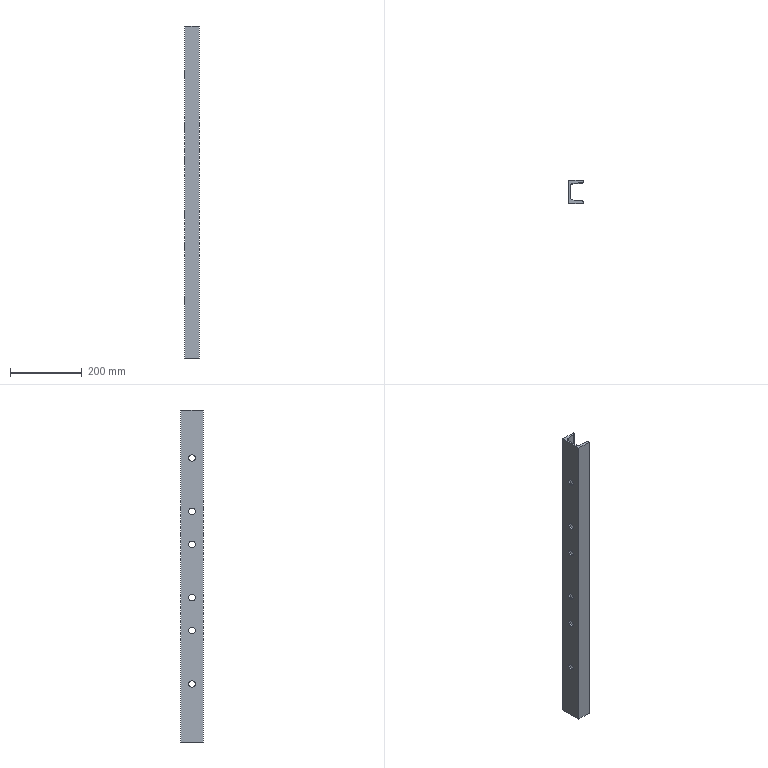Part | STEP file | 750038456 | 1 solid | 26 faces | box 40 x 63 x 924 mm | volume 773051 mm3 | cylinder 16 | plane 10 | commonest cylinder face diameters 18 x12 7.6 x2 15 x2
STEP:
#1=CARTESIAN_POINT('',(4.8,31.5,170.754));
#2=VERTEX_POINT('',#1);
#3=CARTESIAN_POINT('',(4.8,31.5,188.754));
#4=VERTEX_POINT('',#3);
#5=CARTESIAN_POINT('',(4.8,31.5,179.754));
#6=DIRECTION('',(-1.,0.,0.));
#7=DIRECTION('',(0.,0.,1.));
#8=AXIS2_PLACEMENT_3D('',#5,#6,#7);
#9=CIRCLE('',#8,9.);
#10=EDGE_CURVE('',#2,#4,#9,.T.);
#11=ORIENTED_EDGE('',*,*,#10,.F.);
#12=CARTESIAN_POINT('',(0.,31.5,170.754));
#13=VERTEX_POINT('',#12);
#14=CARTESIAN_POINT('',(44.,31.5,170.754));
#15=DIRECTION('',(-1.,0.,0.));
#16=VECTOR('',#15,1000.);
#17=LINE('',#14,#16);
#18=EDGE_CURVE('',#2,#13,#17,.T.);
#19=ORIENTED_EDGE('',*,*,#18,.T.);
#20=CARTESIAN_POINT('',(0.,31.5,188.754));
#21=VERTEX_POINT('',#20);
#22=CARTESIAN_POINT('',(0.,31.5,179.754));
#23=DIRECTION('',(-1.,0.,0.));
#24=DIRECTION('',(0.,0.,1.));
#25=AXIS2_PLACEMENT_3D('',#22,#23,#24);
#26=CIRCLE('',#25,9.);
#27=EDGE_CURVE('',#13,#21,#26,.T.);
#28=ORIENTED_EDGE('',*,*,#27,.T.);
#29=CARTESIAN_POINT('',(44.,31.5,188.754));
#30=DIRECTION('',(-1.,0.,0.));
#31=VECTOR('',#30,1000.);
#32=LINE('',#29,#31);
#33=EDGE_CURVE('',#4,#21,#32,.T.);
#34=ORIENTED_EDGE('',*,*,#33,.F.);
#35=EDGE_LOOP('',(#11,#19,#28,#34));
#36=FACE_OUTER_BOUND('',#35,.T.);
#37=CARTESIAN_POINT('',(44.,31.5,179.754));
#38=DIRECTION('',(-1.,0.,0.));
#39=DIRECTION('',(0.,0.,1.));
#40=AXIS2_PLACEMENT_3D('',#37,#38,#39);
#41=CYLINDRICAL_SURFACE('',#40,9.);
#42=ADVANCED_FACE('',(#36),#41,.F.);
#43=CARTESIAN_POINT('',(4.8,31.5,79.246));
#44=VERTEX_POINT('',#43);
#45=CARTESIAN_POINT('',(4.8,31.5,97.246));
#46=VERTEX_POINT('',#45);
#47=CARTESIAN_POINT('',(4.8,31.5,88.246));
#48=DIRECTION('',(-1.,0.,0.));
#49=DIRECTION('',(0.,0.,1.));
#50=AXIS2_PLACEMENT_3D('',#47,#48,#49);
#51=CIRCLE('',#50,9.);
#52=EDGE_CURVE('',#44,#46,#51,.T.);
#53=ORIENTED_EDGE('',*,*,#52,.F.);
#54=CARTESIAN_POINT('',(0.,31.5,79.246));
#55=VERTEX_POINT('',#54);
#56=CARTESIAN_POINT('',(44.,31.5,79.246));
#57=DIRECTION('',(-1.,0.,0.));
#58=VECTOR('',#57,1000.);
#59=LINE('',#56,#58);
#60=EDGE_CURVE('',#44,#55,#59,.T.);
#61=ORIENTED_EDGE('',*,*,#60,.T.);
#62=CARTESIAN_POINT('',(0.,31.5,97.246));
#63=VERTEX_POINT('',#62);
#64=CARTESIAN_POINT('',(0.,31.5,88.246));
#65=DIRECTION('',(-1.,0.,0.));
#66=DIRECTION('',(0.,0.,1.));
#67=AXIS2_PLACEMENT_3D('',#64,#65,#66);
#68=CIRCLE('',#67,9.);
#69=EDGE_CURVE('',#55,#63,#68,.T.);
#70=ORIENTED_EDGE('',*,*,#69,.T.);
#71=CARTESIAN_POINT('',(44.,31.5,97.246));
#72=DIRECTION('',(-1.,0.,0.));
#73=VECTOR('',#72,1000.);
#74=LINE('',#71,#73);
#75=EDGE_CURVE('',#46,#63,#74,.T.);
#76=ORIENTED_EDGE('',*,*,#75,.F.);
#77=EDGE_LOOP('',(#53,#61,#70,#76));
#78=FACE_OUTER_BOUND('',#77,.T.);
#79=CARTESIAN_POINT('',(44.,31.5,88.246));
#80=DIRECTION('',(-1.,0.,0.));
#81=DIRECTION('',(0.,0.,1.));
#82=AXIS2_PLACEMENT_3D('',#79,#80,#81);
#83=CYLINDRICAL_SURFACE('',#82,9.);
#84=ADVANCED_FACE('',(#78),#83,.F.);
#85=CARTESIAN_POINT('',(4.8,31.5,-160.754));
#86=VERTEX_POINT('',#85);
#87=CARTESIAN_POINT('',(4.8,31.5,-142.754));
#88=VERTEX_POINT('',#87);
#89=CARTESIAN_POINT('',(4.8,31.5,-151.754));
#90=DIRECTION('',(-1.,0.,0.));
#91=DIRECTION('',(0.,0.,1.));
#92=AXIS2_PLACEMENT_3D('',#89,#90,#91);
#93=CIRCLE('',#92,9.);
#94=EDGE_CURVE('',#86,#88,#93,.T.);
#95=ORIENTED_EDGE('',*,*,#94,.F.);
#96=CARTESIAN_POINT('',(0.,31.5,-160.754));
#97=VERTEX_POINT('',#96);
#98=CARTESIAN_POINT('',(44.,31.5,-160.754));
#99=DIRECTION('',(-1.,0.,0.));
#100=VECTOR('',#99,1000.);
#101=LINE('',#98,#100);
#102=EDGE_CURVE('',#86,#97,#101,.T.);
#103=ORIENTED_EDGE('',*,*,#102,.T.);
#104=CARTESIAN_POINT('',(0.,31.5,-142.754));
#105=VERTEX_POINT('',#104);
#106=CARTESIAN_POINT('',(0.,31.5,-151.754));
#107=DIRECTION('',(-1.,0.,0.));
#108=DIRECTION('',(0.,0.,1.));
#109=AXIS2_PLACEMENT_3D('',#106,#107,#108);
#110=CIRCLE('',#109,9.);
#111=EDGE_CURVE('',#97,#105,#110,.T.);
#112=ORIENTED_EDGE('',*,*,#111,.T.);
#113=CARTESIAN_POINT('',(44.,31.5,-142.754));
#114=DIRECTION('',(-1.,0.,0.));
#115=VECTOR('',#114,1000.);
#116=LINE('',#113,#115);
#117=EDGE_CURVE('',#88,#105,#116,.T.);
#118=ORIENTED_EDGE('',*,*,#117,.F.);
#119=EDGE_LOOP('',(#95,#103,#112,#118));
#120=FACE_OUTER_BOUND('',#119,.T.);
#121=CARTESIAN_POINT('',(44.,31.5,-151.754));
#122=DIRECTION('',(-1.,0.,0.));
#123=DIRECTION('',(0.,0.,1.));
#124=AXIS2_PLACEMENT_3D('',#121,#122,#123);
#125=CYLINDRICAL_SURFACE('',#124,9.);
#126=ADVANCED_FACE('',(#120),#125,.F.);
#127=CARTESIAN_POINT('',(4.8,31.5,-309.246));
#128=VERTEX_POINT('',#127);
#129=CARTESIAN_POINT('',(4.8,31.5,-291.246));
#130=VERTEX_POINT('',#129);
#131=CARTESIAN_POINT('',(4.8,31.5,-300.246));
#132=DIRECTION('',(-1.,0.,0.));
#133=DIRECTION('',(0.,0.,1.));
#134=AXIS2_PLACEMENT_3D('',#131,#132,#133);
#135=CIRCLE('',#134,9.);
#136=EDGE_CURVE('',#128,#130,#135,.T.);
#137=ORIENTED_EDGE('',*,*,#136,.F.);
#138=CARTESIAN_POINT('',(0.,31.5,-309.246));
#139=VERTEX_POINT('',#138);
#140=CARTESIAN_POINT('',(44.,31.5,-309.246));
#141=DIRECTION('',(-1.,0.,0.));
#142=VECTOR('',#141,1000.);
#143=LINE('',#140,#142);
#144=EDGE_CURVE('',#128,#139,#143,.T.);
#145=ORIENTED_EDGE('',*,*,#144,.T.);
#146=CARTESIAN_POINT('',(0.,31.5,-291.246));
#147=VERTEX_POINT('',#146);
#148=CARTESIAN_POINT('',(0.,31.5,-300.246));
#149=DIRECTION('',(-1.,0.,0.));
#150=DIRECTION('',(0.,0.,1.));
#151=AXIS2_PLACEMENT_3D('',#148,#149,#150);
#152=CIRCLE('',#151,9.);
#153=EDGE_CURVE('',#139,#147,#152,.T.);
#154=ORIENTED_EDGE('',*,*,#153,.T.);
#155=CARTESIAN_POINT('',(44.,31.5,-291.246));
#156=DIRECTION('',(-1.,0.,0.));
#157=VECTOR('',#156,1000.);
#158=LINE('',#155,#157);
#159=EDGE_CURVE('',#130,#147,#158,.T.);
#160=ORIENTED_EDGE('',*,*,#159,.F.);
#161=EDGE_LOOP('',(#137,#145,#154,#160));
#162=FACE_OUTER_BOUND('',#161,.T.);
#163=CARTESIAN_POINT('',(44.,31.5,-300.246));
#164=DIRECTION('',(-1.,0.,0.));
#165=DIRECTION('',(0.,0.,1.));
#166=AXIS2_PLACEMENT_3D('',#163,#164,#165);
#167=CYLINDRICAL_SURFACE('',#166,9.);
#168=ADVANCED_FACE('',(#162),#167,.F.);
#169=CARTESIAN_POINT('',(4.8,31.5,-69.246));
#170=VERTEX_POINT('',#169);
#171=CARTESIAN_POINT('',(4.8,31.5,-51.246));
#172=VERTEX_POINT('',#171);
#173=CARTESIAN_POINT('',(4.8,31.5,-60.246));
#174=DIRECTION('',(-1.,0.,0.));
#175=DIRECTION('',(0.,0.,1.));
#176=AXIS2_PLACEMENT_3D('',#173,#174,#175);
#177=CIRCLE('',#176,9.);
#178=EDGE_CURVE('',#170,#172,#177,.T.);
#179=ORIENTED_EDGE('',*,*,#178,.F.);
#180=CARTESIAN_POINT('',(0.,31.5,-69.246));
#181=VERTEX_POINT('',#180);
#182=CARTESIAN_POINT('',(44.,31.5,-69.246));
#183=DIRECTION('',(-1.,0.,0.));
#184=VECTOR('',#183,1000.);
#185=LINE('',#182,#184);
#186=EDGE_CURVE('',#170,#181,#185,.T.);
#187=ORIENTED_EDGE('',*,*,#186,.T.);
#188=CARTESIAN_POINT('',(0.,31.5,-51.246));
#189=VERTEX_POINT('',#188);
#190=CARTESIAN_POINT('',(0.,31.5,-60.246));
#191=DIRECTION('',(-1.,0.,0.));
#192=DIRECTION('',(0.,0.,1.));
#193=AXIS2_PLACEMENT_3D('',#190,#191,#192);
#194=CIRCLE('',#193,9.);
#195=EDGE_CURVE('',#181,#189,#194,.T.);
#196=ORIENTED_EDGE('',*,*,#195,.T.);
#197=CARTESIAN_POINT('',(44.,31.5,-51.246));
#198=DIRECTION('',(-1.,0.,0.));
#199=VECTOR('',#198,1000.);
#200=LINE('',#197,#199);
#201=EDGE_CURVE('',#172,#189,#200,.T.);
#202=ORIENTED_EDGE('',*,*,#201,.F.);
#203=EDGE_LOOP('',(#179,#187,#196,#202));
#204=FACE_OUTER_BOUND('',#203,.T.);
#205=CARTESIAN_POINT('',(44.,31.5,-60.246));
#206=DIRECTION('',(-1.,0.,0.));
#207=DIRECTION('',(0.,0.,1.));
#208=AXIS2_PLACEMENT_3D('',#205,#206,#207);
#209=CYLINDRICAL_SURFACE('',#208,9.);
#210=ADVANCED_FACE('',(#204),#209,.F.);
#211=CARTESIAN_POINT('',(4.8,31.5,319.246));
#212=VERTEX_POINT('',#211);
#213=CARTESIAN_POINT('',(4.8,31.5,337.246));
#214=VERTEX_POINT('',#213);
#215=CARTESIAN_POINT('',(4.8,31.5,328.246));
#216=DIRECTION('',(-1.,0.,0.));
#217=DIRECTION('',(0.,0.,1.));
#218=AXIS2_PLACEMENT_3D('',#215,#216,#217);
#219=CIRCLE('',#218,9.);
#220=EDGE_CURVE('',#212,#214,#219,.T.);
#221=ORIENTED_EDGE('',*,*,#220,.F.);
#222=CARTESIAN_POINT('',(0.,31.5,319.246));
#223=VERTEX_POINT('',#222);
#224=CARTESIAN_POINT('',(44.,31.5,319.246));
#225=DIRECTION('',(-1.,0.,0.));
#226=VECTOR('',#225,1000.);
#227=LINE('',#224,#226);
#228=EDGE_CURVE('',#212,#223,#227,.T.);
#229=ORIENTED_EDGE('',*,*,#228,.T.);
#230=CARTESIAN_POINT('',(0.,31.5,337.246));
#231=VERTEX_POINT('',#230);
#232=CARTESIAN_POINT('',(0.,31.5,328.246));
#233=DIRECTION('',(-1.,0.,0.));
#234=DIRECTION('',(0.,0.,1.));
#235=AXIS2_PLACEMENT_3D('',#232,#233,#234);
#236=CIRCLE('',#235,9.);
#237=EDGE_CURVE('',#223,#231,#236,.T.);
#238=ORIENTED_EDGE('',*,*,#237,.T.);
#239=CARTESIAN_POINT('',(44.,31.5,337.246));
#240=DIRECTION('',(-1.,0.,0.));
#241=VECTOR('',#240,1000.);
#242=LINE('',#239,#241);
#243=EDGE_CURVE('',#214,#231,#242,.T.);
#244=ORIENTED_EDGE('',*,*,#243,.F.);
#245=EDGE_LOOP('',(#221,#229,#238,#244));
#246=FACE_OUTER_BOUND('',#245,.T.);
#247=CARTESIAN_POINT('',(44.,31.5,328.246));
#248=DIRECTION('',(-1.,0.,0.));
#249=DIRECTION('',(0.,0.,1.));
#250=AXIS2_PLACEMENT_3D('',#247,#248,#249);
#251=CYLINDRICAL_SURFACE('',#250,9.);
#252=ADVANCED_FACE('',(#246),#251,.F.);
#253=CARTESIAN_POINT('',(0.,0.,462.));
#254=VERTEX_POINT('',#253);
#255=CARTESIAN_POINT('',(0.,0.,-462.));
#256=VERTEX_POINT('',#255);
#257=CARTESIAN_POINT('',(0.,0.,462.));
#258=DIRECTION('',(0.,0.,-1.));
#259=VECTOR('',#258,1000.);
#260=LINE('',#257,#259);
#261=EDGE_CURVE('',#254,#256,#260,.T.);
#262=ORIENTED_EDGE('',*,*,#261,.F.);
#263=CARTESIAN_POINT('',(0.,63.,462.));
#264=VERTEX_POINT('',#263);
#265=CARTESIAN_POINT('',(0.,63.,462.));
#266=DIRECTION('',(0.,-1.,0.));
#267=VECTOR('',#266,1000.);
#268=LINE('',#265,#267);
#269=EDGE_CURVE('',#264,#254,#268,.T.);
#270=ORIENTED_EDGE('',*,*,#269,.F.);
#271=CARTESIAN_POINT('',(0.,63.,-462.));
#272=VERTEX_POINT('',#271);
#273=CARTESIAN_POINT('',(0.,63.,462.));
#274=DIRECTION('',(0.,0.,1.));
#275=VECTOR('',#274,1000.);
#276=LINE('',#273,#275);
#277=EDGE_CURVE('',#272,#264,#276,.T.);
#278=ORIENTED_EDGE('',*,*,#277,.F.);
#279=CARTESIAN_POINT('',(0.,63.,-462.));
#280=DIRECTION('',(0.,1.,0.));
#281=VECTOR('',#280,1000.);
#282=LINE('',#279,#281);
#283=EDGE_CURVE('',#256,#272,#282,.T.);
#284=ORIENTED_EDGE('',*,*,#283,.F.);
#285=EDGE_LOOP('',(#262,#270,#278,#284));
#286=FACE_OUTER_BOUND('',#285,.T.);
#287=CARTESIAN_POINT('',(0.,31.5,179.754));
#288=DIRECTION('',(-1.,0.,0.));
#289=DIRECTION('',(0.,0.,1.));
#290=AXIS2_PLACEMENT_3D('',#287,#288,#289);
#291=CIRCLE('',#290,9.);
#292=EDGE_CURVE('',#21,#13,#291,.T.);
#293=ORIENTED_EDGE('',*,*,#292,.F.);
#294=ORIENTED_EDGE('',*,*,#27,.F.);
#295=EDGE_LOOP('',(#293,#294));
#296=FACE_BOUND('',#295,.T.);
#297=CARTESIAN_POINT('',(0.,31.5,88.246));
#298=DIRECTION('',(-1.,0.,0.));
#299=DIRECTION('',(0.,0.,1.));
#300=AXIS2_PLACEMENT_3D('',#297,#298,#299);
#301=CIRCLE('',#300,9.);
#302=EDGE_CURVE('',#63,#55,#301,.T.);
#303=ORIENTED_EDGE('',*,*,#302,.F.);
#304=ORIENTED_EDGE('',*,*,#69,.F.);
#305=EDGE_LOOP('',(#303,#304));
#306=FACE_BOUND('',#305,.T.);
#307=CARTESIAN_POINT('',(0.,31.5,-151.754));
#308=DIRECTION('',(-1.,0.,0.));
#309=DIRECTION('',(0.,0.,1.));
#310=AXIS2_PLACEMENT_3D('',#307,#308,#309);
#311=CIRCLE('',#310,9.);
#312=EDGE_CURVE('',#105,#97,#311,.T.);
#313=ORIENTED_EDGE('',*,*,#312,.F.);
#314=ORIENTED_EDGE('',*,*,#111,.F.);
#315=EDGE_LOOP('',(#313,#314));
#316=FACE_BOUND('',#315,.T.);
#317=CARTESIAN_POINT('',(0.,31.5,-300.246));
#318=DIRECTION('',(-1.,0.,0.));
#319=DIRECTION('',(0.,0.,1.));
#320=AXIS2_PLACEMENT_3D('',#317,#318,#319);
#321=CIRCLE('',#320,9.);
#322=EDGE_CURVE('',#147,#139,#321,.T.);
#323=ORIENTED_EDGE('',*,*,#322,.F.);
#324=ORIENTED_EDGE('',*,*,#153,.F.);
#325=EDGE_LOOP('',(#323,#324));
#326=FACE_BOUND('',#325,.T.);
#327=CARTESIAN_POINT('',(0.,31.5,-60.246));
#328=DIRECTION('',(-1.,0.,0.));
#329=DIRECTION('',(0.,0.,1.));
#330=AXIS2_PLACEMENT_3D('',#327,#328,#329);
#331=CIRCLE('',#330,9.);
#332=EDGE_CURVE('',#189,#181,#331,.T.);
#333=ORIENTED_EDGE('',*,*,#332,.F.);
#334=ORIENTED_EDGE('',*,*,#195,.F.);
#335=EDGE_LOOP('',(#333,#334));
#336=FACE_BOUND('',#335,.T.);
#337=CARTESIAN_POINT('',(0.,31.5,328.246));
#338=DIRECTION('',(-1.,0.,0.));
#339=DIRECTION('',(0.,0.,1.));
#340=AXIS2_PLACEMENT_3D('',#337,#338,#339);
#341=CIRCLE('',#340,9.);
#342=EDGE_CURVE('',#231,#223,#341,.T.);
#343=ORIENTED_EDGE('',*,*,#342,.F.);
#344=ORIENTED_EDGE('',*,*,#237,.F.);
#345=EDGE_LOOP('',(#343,#344));
#346=FACE_BOUND('',#345,.T.);
#347=CARTESIAN_POINT('',(0.,63.,462.));
#348=DIRECTION('',(1.,0.,0.));
#349=DIRECTION('',(0.,0.,-1.));
#350=AXIS2_PLACEMENT_3D('',#347,#348,#349);
#351=PLANE('',#350);
#352=ADVANCED_FACE('',(#286,#296,#306,#316,#326,#336,#346),#351,.F.);
#353=CARTESIAN_POINT('',(40.,63.,-462.));
#354=VERTEX_POINT('',#353);
#355=CARTESIAN_POINT('',(36.2,63.,-462.));
#356=DIRECTION('',(-1.,0.,0.));
#357=VECTOR('',#356,1000.);
#358=LINE('',#355,#357);
#359=EDGE_CURVE('',#354,#272,#358,.T.);
#360=ORIENTED_EDGE('',*,*,#359,.F.);
#361=CARTESIAN_POINT('',(40.,60.699,-462.));
#362=VERTEX_POINT('',#361);
#363=CARTESIAN_POINT('',(40.,2.301,-462.));
#364=DIRECTION('',(0.,1.,0.));
#365=VECTOR('',#364,1000.);
#366=LINE('',#363,#365);
#367=EDGE_CURVE('',#362,#354,#366,.T.);
#368=ORIENTED_EDGE('',*,*,#367,.F.);
#369=CARTESIAN_POINT('',(36.578,56.918,-462.));
#370=VERTEX_POINT('',#369);
#371=CARTESIAN_POINT('',(36.2,60.699,-462.));
#372=DIRECTION('',(0.,0.,1.));
#373=DIRECTION('',(-1.,0.,0.));
#374=AXIS2_PLACEMENT_3D('',#371,#372,#373);
#375=CIRCLE('',#374,3.8);
#376=EDGE_CURVE('',#370,#362,#375,.T.);
#377=ORIENTED_EDGE('',*,*,#376,.F.);
#378=CARTESIAN_POINT('',(11.554,54.415,-462.));
#379=VERTEX_POINT('',#378);
#380=CARTESIAN_POINT('',(11.554,54.415,-462.));
#381=DIRECTION('',(0.995,0.0995,0.));
#382=VECTOR('',#381,1000.);
#383=LINE('',#380,#382);
#384=EDGE_CURVE('',#379,#370,#383,.T.);
#385=ORIENTED_EDGE('',*,*,#384,.F.);
#386=CARTESIAN_POINT('',(4.8,46.953,-462.));
#387=VERTEX_POINT('',#386);
#388=CARTESIAN_POINT('',(12.3,46.953,-462.));
#389=DIRECTION('',(0.,0.,-1.));
#390=DIRECTION('',(-1.,0.,0.));
#391=AXIS2_PLACEMENT_3D('',#388,#389,#390);
#392=CIRCLE('',#391,7.5);
#393=EDGE_CURVE('',#387,#379,#392,.T.);
#394=ORIENTED_EDGE('',*,*,#393,.F.);
#395=CARTESIAN_POINT('',(4.8,16.047,-462.));
#396=VERTEX_POINT('',#395);
#397=CARTESIAN_POINT('',(4.8,2.301,-462.));
#398=DIRECTION('',(0.,1.,0.));
#399=VECTOR('',#398,1000.);
#400=LINE('',#397,#399);
#401=EDGE_CURVE('',#396,#387,#400,.T.);
#402=ORIENTED_EDGE('',*,*,#401,.F.);
#403=CARTESIAN_POINT('',(11.554,8.585,-462.));
#404=VERTEX_POINT('',#403);
#405=CARTESIAN_POINT('',(12.3,16.047,-462.));
#406=DIRECTION('',(0.,0.,-1.));
#407=DIRECTION('',(-1.,0.,0.));
#408=AXIS2_PLACEMENT_3D('',#405,#406,#407);
#409=CIRCLE('',#408,7.5);
#410=EDGE_CURVE('',#404,#396,#409,.T.);
#411=ORIENTED_EDGE('',*,*,#410,.F.);
#412=CARTESIAN_POINT('',(36.578,6.082,-462.));
#413=VERTEX_POINT('',#412);
#414=CARTESIAN_POINT('',(36.578,6.082,-462.));
#415=DIRECTION('',(-0.995,0.0995,0.));
#416=VECTOR('',#415,1000.);
#417=LINE('',#414,#416);
#418=EDGE_CURVE('',#413,#404,#417,.T.);
#419=ORIENTED_EDGE('',*,*,#418,.F.);
#420=CARTESIAN_POINT('',(40.,2.301,-462.));
#421=VERTEX_POINT('',#420);
#422=CARTESIAN_POINT('',(36.2,2.301,-462.));
#423=DIRECTION('',(0.,0.,1.));
#424=DIRECTION('',(-1.,0.,0.));
#425=AXIS2_PLACEMENT_3D('',#422,#423,#424);
#426=CIRCLE('',#425,3.8);
#427=EDGE_CURVE('',#421,#413,#426,.T.);
#428=ORIENTED_EDGE('',*,*,#427,.F.);
#429=CARTESIAN_POINT('',(40.,0.,-462.));
#430=VERTEX_POINT('',#429);
#431=CARTESIAN_POINT('',(40.,2.301,-462.));
#432=DIRECTION('',(0.,1.,0.));
#433=VECTOR('',#432,1000.);
#434=LINE('',#431,#433);
#435=EDGE_CURVE('',#430,#421,#434,.T.);
#436=ORIENTED_EDGE('',*,*,#435,.F.);
#437=CARTESIAN_POINT('',(36.2,0.,-462.));
#438=DIRECTION('',(1.,0.,0.));
#439=VECTOR('',#438,1000.);
#440=LINE('',#437,#439);
#441=EDGE_CURVE('',#256,#430,#440,.T.);
#442=ORIENTED_EDGE('',*,*,#441,.F.);
#443=ORIENTED_EDGE('',*,*,#283,.T.);
#444=EDGE_LOOP('',(#360,#368,#377,#385,#394,#402,#411,#419,#428,#436,#442,#443));
#445=FACE_OUTER_BOUND('',#444,.T.);
#446=CARTESIAN_POINT('',(36.2,2.301,-462.));
#447=DIRECTION('',(0.,0.,1.));
#448=DIRECTION('',(1.,0.,0.));
#449=AXIS2_PLACEMENT_3D('',#446,#447,#448);
#450=PLANE('',#449);
#451=ADVANCED_FACE('',(#445),#450,.F.);
#452=CARTESIAN_POINT('',(40.,0.,462.));
#453=VERTEX_POINT('',#452);
#454=CARTESIAN_POINT('',(40.,0.,462.));
#455=DIRECTION('',(0.,0.,-1.));
#456=VECTOR('',#455,1000.);
#457=LINE('',#454,#456);
#458=EDGE_CURVE('',#453,#430,#457,.T.);
#459=ORIENTED_EDGE('',*,*,#458,.F.);
#460=CARTESIAN_POINT('',(0.,0.,462.));
#461=DIRECTION('',(1.,0.,0.));
#462=VECTOR('',#461,1000.);
#463=LINE('',#460,#462);
#464=EDGE_CURVE('',#254,#453,#463,.T.);
#465=ORIENTED_EDGE('',*,*,#464,.F.);
#466=ORIENTED_EDGE('',*,*,#261,.T.);
#467=ORIENTED_EDGE('',*,*,#441,.T.);
#468=EDGE_LOOP('',(#459,#465,#466,#467));
#469=FACE_OUTER_BOUND('',#468,.T.);
#470=CARTESIAN_POINT('',(0.,0.,462.));
#471=DIRECTION('',(0.,1.,0.));
#472=DIRECTION('',(0.,0.,1.));
#473=AXIS2_PLACEMENT_3D('',#470,#471,#472);
#474=PLANE('',#473);
#475=ADVANCED_FACE('',(#469),#474,.F.);
#476=CARTESIAN_POINT('',(40.,60.699,462.));
#477=VERTEX_POINT('',#476);
#478=CARTESIAN_POINT('',(40.,63.,462.));
#479=VERTEX_POINT('',#478);
#480=CARTESIAN_POINT('',(40.,2.301,462.));
#481=DIRECTION('',(0.,1.,0.));
#482=VECTOR('',#481,1000.);
#483=LINE('',#480,#482);
#484=EDGE_CURVE('',#477,#479,#483,.T.);
#485=ORIENTED_EDGE('',*,*,#484,.T.);
#486=CARTESIAN_POINT('',(36.2,63.,462.));
#487=DIRECTION('',(-1.,0.,0.));
#488=VECTOR('',#487,1000.);
#489=LINE('',#486,#488);
#490=EDGE_CURVE('',#479,#264,#489,.T.);
#491=ORIENTED_EDGE('',*,*,#490,.T.);
#492=ORIENTED_EDGE('',*,*,#269,.T.);
#493=ORIENTED_EDGE('',*,*,#464,.T.);
#494=CARTESIAN_POINT('',(40.,2.301,462.));
#495=VERTEX_POINT('',#494);
#496=CARTESIAN_POINT('',(40.,2.301,462.));
#497=DIRECTION('',(0.,1.,0.));
#498=VECTOR('',#497,1000.);
#499=LINE('',#496,#498);
#500=EDGE_CURVE('',#453,#495,#499,.T.);
#501=ORIENTED_EDGE('',*,*,#500,.T.);
#502=CARTESIAN_POINT('',(36.578,6.082,462.));
#503=VERTEX_POINT('',#502);
#504=CARTESIAN_POINT('',(36.2,2.301,462.));
#505=DIRECTION('',(0.,0.,1.));
#506=DIRECTION('',(-1.,0.,0.));
#507=AXIS2_PLACEMENT_3D('',#504,#505,#506);
#508=CIRCLE('',#507,3.8);
#509=EDGE_CURVE('',#495,#503,#508,.T.);
#510=ORIENTED_EDGE('',*,*,#509,.T.);
#511=CARTESIAN_POINT('',(11.554,8.585,462.));
#512=VERTEX_POINT('',#511);
#513=CARTESIAN_POINT('',(36.578,6.082,462.));
#514=DIRECTION('',(-0.995,0.0995,0.));
#515=VECTOR('',#514,1000.);
#516=LINE('',#513,#515);
#517=EDGE_CURVE('',#503,#512,#516,.T.);
#518=ORIENTED_EDGE('',*,*,#517,.T.);
#519=CARTESIAN_POINT('',(4.8,16.047,462.));
#520=VERTEX_POINT('',#519);
#521=CARTESIAN_POINT('',(12.3,16.047,462.));
#522=DIRECTION('',(0.,0.,-1.));
#523=DIRECTION('',(-1.,0.,0.));
#524=AXIS2_PLACEMENT_3D('',#521,#522,#523);
#525=CIRCLE('',#524,7.5);
#526=EDGE_CURVE('',#512,#520,#525,.T.);
#527=ORIENTED_EDGE('',*,*,#526,.T.);
#528=CARTESIAN_POINT('',(4.8,46.953,462.));
#529=VERTEX_POINT('',#528);
#530=CARTESIAN_POINT('',(4.8,2.301,462.));
#531=DIRECTION('',(0.,1.,0.));
#532=VECTOR('',#531,1000.);
#533=LINE('',#530,#532);
#534=EDGE_CURVE('',#520,#529,#533,.T.);
#535=ORIENTED_EDGE('',*,*,#534,.T.);
#536=CARTESIAN_POINT('',(11.554,54.415,462.));
#537=VERTEX_POINT('',#536);
#538=CARTESIAN_POINT('',(12.3,46.953,462.));
#539=DIRECTION('',(0.,0.,-1.));
#540=DIRECTION('',(-1.,0.,0.));
#541=AXIS2_PLACEMENT_3D('',#538,#539,#540);
#542=CIRCLE('',#541,7.5);
#543=EDGE_CURVE('',#529,#537,#542,.T.);
#544=ORIENTED_EDGE('',*,*,#543,.T.);
#545=CARTESIAN_POINT('',(36.578,56.918,462.));
#546=VERTEX_POINT('',#545);
#547=CARTESIAN_POINT('',(11.554,54.415,462.));
#548=DIRECTION('',(0.995,0.0995,0.));
#549=VECTOR('',#548,1000.);
#550=LINE('',#547,#549);
#551=EDGE_CURVE('',#537,#546,#550,.T.);
#552=ORIENTED_EDGE('',*,*,#551,.T.);
#553=CARTESIAN_POINT('',(36.2,60.699,462.));
#554=DIRECTION('',(0.,0.,1.));
#555=DIRECTION('',(-1.,0.,0.));
#556=AXIS2_PLACEMENT_3D('',#553,#554,#555);
#557=CIRCLE('',#556,3.8);
#558=EDGE_CURVE('',#546,#477,#557,.T.);
#559=ORIENTED_EDGE('',*,*,#558,.T.);
#560=EDGE_LOOP('',(#485,#491,#492,#493,#501,#510,#518,#527,#535,#544,#552,#559));
#561=FACE_OUTER_BOUND('',#560,.T.);
#562=CARTESIAN_POINT('',(36.2,2.301,462.));
#563=DIRECTION('',(0.,0.,1.));
#564=DIRECTION('',(1.,0.,0.));
#565=AXIS2_PLACEMENT_3D('',#562,#563,#564);
#566=PLANE('',#565);
#567=ADVANCED_FACE('',(#561),#566,.T.);
#568=ORIENTED_EDGE('',*,*,#277,.T.);
#569=ORIENTED_EDGE('',*,*,#490,.F.);
#570=CARTESIAN_POINT('',(40.,63.,462.));
#571=DIRECTION('',(0.,0.,1.));
#572=VECTOR('',#571,1000.);
#573=LINE('',#570,#572);
#574=EDGE_CURVE('',#354,#479,#573,.T.);
#575=ORIENTED_EDGE('',*,*,#574,.F.);
#576=ORIENTED_EDGE('',*,*,#359,.T.);
#577=EDGE_LOOP('',(#568,#569,#575,#576));
#578=FACE_OUTER_BOUND('',#577,.T.);
#579=CARTESIAN_POINT('',(40.,63.,462.));
#580=DIRECTION('',(0.,-1.,0.));
#581=DIRECTION('',(0.,0.,-1.));
#582=AXIS2_PLACEMENT_3D('',#579,#580,#581);
#583=PLANE('',#582);
#584=ADVANCED_FACE('',(#578),#583,.F.);
#585=ORIENTED_EDGE('',*,*,#18,.F.);
#586=CARTESIAN_POINT('',(4.8,31.5,179.754));
#587=DIRECTION('',(-1.,0.,0.));
#588=DIRECTION('',(0.,0.,1.));
#589=AXIS2_PLACEMENT_3D('',#586,#587,#588);
#590=CIRCLE('',#589,9.);
#591=EDGE_CURVE('',#4,#2,#590,.T.);
#592=ORIENTED_EDGE('',*,*,#591,.F.);
#593=ORIENTED_EDGE('',*,*,#33,.T.);
#594=ORIENTED_EDGE('',*,*,#292,.T.);
#595=EDGE_LOOP('',(#585,#592,#593,#594));
#596=FACE_OUTER_BOUND('',#595,.T.);
#597=CARTESIAN_POINT('',(44.,31.5,179.754));
#598=DIRECTION('',(-1.,0.,0.));
#599=DIRECTION('',(0.,0.,1.));
#600=AXIS2_PLACEMENT_3D('',#597,#598,#599);
#601=CYLINDRICAL_SURFACE('',#600,9.);
#602=ADVANCED_FACE('',(#596),#601,.F.);
#603=ORIENTED_EDGE('',*,*,#60,.F.);
#604=CARTESIAN_POINT('',(4.8,31.5,88.246));
#605=DIRECTION('',(-1.,0.,0.));
#606=DIRECTION('',(0.,0.,1.));
#607=AXIS2_PLACEMENT_3D('',#604,#605,#606);
#608=CIRCLE('',#607,9.);
#609=EDGE_CURVE('',#46,#44,#608,.T.);
#610=ORIENTED_EDGE('',*,*,#609,.F.);
#611=ORIENTED_EDGE('',*,*,#75,.T.);
#612=ORIENTED_EDGE('',*,*,#302,.T.);
#613=EDGE_LOOP('',(#603,#610,#611,#612));
#614=FACE_OUTER_BOUND('',#613,.T.);
#615=CARTESIAN_POINT('',(44.,31.5,88.246));
#616=DIRECTION('',(-1.,0.,0.));
#617=DIRECTION('',(0.,0.,1.));
#618=AXIS2_PLACEMENT_3D('',#615,#616,#617);
#619=CYLINDRICAL_SURFACE('',#618,9.);
#620=ADVANCED_FACE('',(#614),#619,.F.);
#621=ORIENTED_EDGE('',*,*,#102,.F.);
#622=CARTESIAN_POINT('',(4.8,31.5,-151.754));
#623=DIRECTION('',(-1.,0.,0.));
#624=DIRECTION('',(0.,0.,1.));
#625=AXIS2_PLACEMENT_3D('',#622,#623,#624);
#626=CIRCLE('',#625,9.);
#627=EDGE_CURVE('',#88,#86,#626,.T.);
#628=ORIENTED_EDGE('',*,*,#627,.F.);
#629=ORIENTED_EDGE('',*,*,#117,.T.);
#630=ORIENTED_EDGE('',*,*,#312,.T.);
#631=EDGE_LOOP('',(#621,#628,#629,#630));
#632=FACE_OUTER_BOUND('',#631,.T.);
#633=CARTESIAN_POINT('',(44.,31.5,-151.754));
#634=DIRECTION('',(-1.,0.,0.));
#635=DIRECTION('',(0.,0.,1.));
#636=AXIS2_PLACEMENT_3D('',#633,#634,#635);
#637=CYLINDRICAL_SURFACE('',#636,9.);
#638=ADVANCED_FACE('',(#632),#637,.F.);
#639=ORIENTED_EDGE('',*,*,#144,.F.);
#640=CARTESIAN_POINT('',(4.8,31.5,-300.246));
#641=DIRECTION('',(-1.,0.,0.));
#642=DIRECTION('',(0.,0.,1.));
#643=AXIS2_PLACEMENT_3D('',#640,#641,#642);
#644=CIRCLE('',#643,9.);
#645=EDGE_CURVE('',#130,#128,#644,.T.);
#646=ORIENTED_EDGE('',*,*,#645,.F.);
#647=ORIENTED_EDGE('',*,*,#159,.T.);
#648=ORIENTED_EDGE('',*,*,#322,.T.);
#649=EDGE_LOOP('',(#639,#646,#647,#648));
#650=FACE_OUTER_BOUND('',#649,.T.);
#651=CARTESIAN_POINT('',(44.,31.5,-300.246));
#652=DIRECTION('',(-1.,0.,0.));
#653=DIRECTION('',(0.,0.,1.));
#654=AXIS2_PLACEMENT_3D('',#651,#652,#653);
#655=CYLINDRICAL_SURFACE('',#654,9.);
#656=ADVANCED_FACE('',(#650),#655,.F.);
#657=ORIENTED_EDGE('',*,*,#186,.F.);
#658=CARTESIAN_POINT('',(4.8,31.5,-60.246));
#659=DIRECTION('',(-1.,0.,0.));
#660=DIRECTION('',(0.,0.,1.));
#661=AXIS2_PLACEMENT_3D('',#658,#659,#660);
#662=CIRCLE('',#661,9.);
#663=EDGE_CURVE('',#172,#170,#662,.T.);
#664=ORIENTED_EDGE('',*,*,#663,.F.);
#665=ORIENTED_EDGE('',*,*,#201,.T.);
#666=ORIENTED_EDGE('',*,*,#332,.T.);
#667=EDGE_LOOP('',(#657,#664,#665,#666));
#668=FACE_OUTER_BOUND('',#667,.T.);
#669=CARTESIAN_POINT('',(44.,31.5,-60.246));
#670=DIRECTION('',(-1.,0.,0.));
#671=DIRECTION('',(0.,0.,1.));
#672=AXIS2_PLACEMENT_3D('',#669,#670,#671);
#673=CYLINDRICAL_SURFACE('',#672,9.);
#674=ADVANCED_FACE('',(#668),#673,.F.);
#675=ORIENTED_EDGE('',*,*,#228,.F.);
#676=CARTESIAN_POINT('',(4.8,31.5,328.246));
#677=DIRECTION('',(-1.,0.,0.));
#678=DIRECTION('',(0.,0.,1.));
#679=AXIS2_PLACEMENT_3D('',#676,#677,#678);
#680=CIRCLE('',#679,9.);
#681=EDGE_CURVE('',#214,#212,#680,.T.);
#682=ORIENTED_EDGE('',*,*,#681,.F.);
#683=ORIENTED_EDGE('',*,*,#243,.T.);
#684=ORIENTED_EDGE('',*,*,#342,.T.);
#685=EDGE_LOOP('',(#675,#682,#683,#684));
#686=FACE_OUTER_BOUND('',#685,.T.);
#687=CARTESIAN_POINT('',(44.,31.5,328.246));
#688=DIRECTION('',(-1.,0.,0.));
#689=DIRECTION('',(0.,0.,1.));
#690=AXIS2_PLACEMENT_3D('',#687,#688,#689);
#691=CYLINDRICAL_SURFACE('',#690,9.);
#692=ADVANCED_FACE('',(#686),#691,.F.);
#693=ORIENTED_EDGE('',*,*,#574,.T.);
#694=ORIENTED_EDGE('',*,*,#484,.F.);
#695=CARTESIAN_POINT('',(40.,60.699,462.));
#696=DIRECTION('',(0.,0.,1.));
#697=VECTOR('',#696,1000.);
#698=LINE('',#695,#697);
#699=EDGE_CURVE('',#362,#477,#698,.T.);
#700=ORIENTED_EDGE('',*,*,#699,.F.);
#701=ORIENTED_EDGE('',*,*,#367,.T.);
#702=EDGE_LOOP('',(#693,#694,#700,#701));
#703=FACE_OUTER_BOUND('',#702,.T.);
#704=CARTESIAN_POINT('',(40.,60.699,462.));
#705=DIRECTION('',(-1.,0.,0.));
#706=DIRECTION('',(0.,-1.,0.));
#707=AXIS2_PLACEMENT_3D('',#704,#705,#706);
#708=PLANE('',#707);
#709=ADVANCED_FACE('',(#703),#708,.F.);
#710=ORIENTED_EDGE('',*,*,#558,.F.);
#711=CARTESIAN_POINT('',(36.578,56.918,462.));
#712=DIRECTION('',(0.,0.,-1.));
#713=VECTOR('',#712,1000.);
#714=LINE('',#711,#713);
#715=EDGE_CURVE('',#546,#370,#714,.T.);
#716=ORIENTED_EDGE('',*,*,#715,.T.);
#717=ORIENTED_EDGE('',*,*,#376,.T.);
#718=ORIENTED_EDGE('',*,*,#699,.T.);
#719=EDGE_LOOP('',(#710,#716,#717,#718));
#720=FACE_OUTER_BOUND('',#719,.T.);
#721=CARTESIAN_POINT('',(36.2,60.699,462.));
#722=DIRECTION('',(0.,0.,-1.));
#723=DIRECTION('',(-1.,0.,0.));
#724=AXIS2_PLACEMENT_3D('',#721,#722,#723);
#725=CYLINDRICAL_SURFACE('',#724,3.8);
#726=ADVANCED_FACE('',(#720),#725,.T.);
#727=ORIENTED_EDGE('',*,*,#715,.F.);
#728=ORIENTED_EDGE('',*,*,#551,.F.);
#729=CARTESIAN_POINT('',(11.554,54.415,462.));
#730=DIRECTION('',(0.,0.,1.));
#731=VECTOR('',#730,1000.);
#732=LINE('',#729,#731);
#733=EDGE_CURVE('',#379,#537,#732,.T.);
#734=ORIENTED_EDGE('',*,*,#733,.F.);
#735=ORIENTED_EDGE('',*,*,#384,.T.);
#736=EDGE_LOOP('',(#727,#728,#734,#735));
#737=FACE_OUTER_BOUND('',#736,.T.);
#738=CARTESIAN_POINT('',(11.554,54.415,462.));
#739=DIRECTION('',(-0.0995,0.995,0.));
#740=DIRECTION('',(-0.995,-0.0995,0.));
#741=AXIS2_PLACEMENT_3D('',#738,#739,#740);
#742=PLANE('',#741);
#743=ADVANCED_FACE('',(#737),#742,.F.);
#744=ORIENTED_EDGE('',*,*,#733,.T.);
#745=ORIENTED_EDGE('',*,*,#543,.F.);
#746=CARTESIAN_POINT('',(4.8,46.953,462.));
#747=DIRECTION('',(0.,0.,1.));
#748=VECTOR('',#747,1000.);
#749=LINE('',#746,#748);
#750=EDGE_CURVE('',#387,#529,#749,.T.);
#751=ORIENTED_EDGE('',*,*,#750,.F.);
#752=ORIENTED_EDGE('',*,*,#393,.T.);
#753=EDGE_LOOP('',(#744,#745,#751,#752));
#754=FACE_OUTER_BOUND('',#753,.T.);
#755=CARTESIAN_POINT('',(12.3,46.953,462.));
#756=DIRECTION('',(0.,0.,-1.));
#757=DIRECTION('',(-1.,0.,0.));
#758=AXIS2_PLACEMENT_3D('',#755,#756,#757);
#759=CYLINDRICAL_SURFACE('',#758,7.5);
#760=ADVANCED_FACE('',(#754),#759,.F.);
#761=ORIENTED_EDGE('',*,*,#750,.T.);
#762=ORIENTED_EDGE('',*,*,#534,.F.);
#763=CARTESIAN_POINT('',(4.8,16.047,462.));
#764=DIRECTION('',(0.,0.,1.));
#765=VECTOR('',#764,1000.);
#766=LINE('',#763,#765);
#767=EDGE_CURVE('',#396,#520,#766,.T.);
#768=ORIENTED_EDGE('',*,*,#767,.F.);
#769=ORIENTED_EDGE('',*,*,#401,.T.);
#770=EDGE_LOOP('',(#761,#762,#768,#769));
#771=FACE_OUTER_BOUND('',#770,.T.);
#772=ORIENTED_EDGE('',*,*,#591,.T.);
#773=ORIENTED_EDGE('',*,*,#10,.T.);
#774=EDGE_LOOP('',(#772,#773));
#775=FACE_BOUND('',#774,.T.);
#776=ORIENTED_EDGE('',*,*,#609,.T.);
#777=ORIENTED_EDGE('',*,*,#52,.T.);
#778=EDGE_LOOP('',(#776,#777));
#779=FACE_BOUND('',#778,.T.);
#780=ORIENTED_EDGE('',*,*,#627,.T.);
#781=ORIENTED_EDGE('',*,*,#94,.T.);
#782=EDGE_LOOP('',(#780,#781));
#783=FACE_BOUND('',#782,.T.);
#784=ORIENTED_EDGE('',*,*,#645,.T.);
#785=ORIENTED_EDGE('',*,*,#136,.T.);
#786=EDGE_LOOP('',(#784,#785));
#787=FACE_BOUND('',#786,.T.);
#788=ORIENTED_EDGE('',*,*,#663,.T.);
#789=ORIENTED_EDGE('',*,*,#178,.T.);
#790=EDGE_LOOP('',(#788,#789));
#791=FACE_BOUND('',#790,.T.);
#792=ORIENTED_EDGE('',*,*,#681,.T.);
#793=ORIENTED_EDGE('',*,*,#220,.T.);
#794=EDGE_LOOP('',(#792,#793));
#795=FACE_BOUND('',#794,.T.);
#796=CARTESIAN_POINT('',(4.8,16.047,462.));
#797=DIRECTION('',(-1.,0.,0.));
#798=DIRECTION('',(0.,-1.,0.));
#799=AXIS2_PLACEMENT_3D('',#796,#797,#798);
#800=PLANE('',#799);
#801=ADVANCED_FACE('',(#771,#775,#779,#783,#787,#791,#795),#800,.F.);
#802=ORIENTED_EDGE('',*,*,#767,.T.);
#803=ORIENTED_EDGE('',*,*,#526,.F.);
#804=CARTESIAN_POINT('',(11.554,8.585,462.));
#805=DIRECTION('',(0.,0.,1.));
#806=VECTOR('',#805,1000.);
#807=LINE('',#804,#806);
#808=EDGE_CURVE('',#404,#512,#807,.T.);
#809=ORIENTED_EDGE('',*,*,#808,.F.);
#810=ORIENTED_EDGE('',*,*,#410,.T.);
#811=EDGE_LOOP('',(#802,#803,#809,#810));
#812=FACE_OUTER_BOUND('',#811,.T.);
#813=CARTESIAN_POINT('',(12.3,16.047,462.));
#814=DIRECTION('',(0.,0.,-1.));
#815=DIRECTION('',(-1.,0.,0.));
#816=AXIS2_PLACEMENT_3D('',#813,#814,#815);
#817=CYLINDRICAL_SURFACE('',#816,7.5);
#818=ADVANCED_FACE('',(#812),#817,.F.);
#819=ORIENTED_EDGE('',*,*,#808,.T.);
#820=ORIENTED_EDGE('',*,*,#517,.F.);
#821=CARTESIAN_POINT('',(36.578,6.082,462.));
#822=DIRECTION('',(0.,0.,1.));
#823=VECTOR('',#822,1000.);
#824=LINE('',#821,#823);
#825=EDGE_CURVE('',#413,#503,#824,.T.);
#826=ORIENTED_EDGE('',*,*,#825,.F.);
#827=ORIENTED_EDGE('',*,*,#418,.T.);
#828=EDGE_LOOP('',(#819,#820,#826,#827));
#829=FACE_OUTER_BOUND('',#828,.T.);
#830=CARTESIAN_POINT('',(36.578,6.082,462.));
#831=DIRECTION('',(-0.0995,-0.995,0.));
#832=DIRECTION('',(0.995,-0.0995,0.));
#833=AXIS2_PLACEMENT_3D('',#830,#831,#832);
#834=PLANE('',#833);
#835=ADVANCED_FACE('',(#829),#834,.F.);
#836=ORIENTED_EDGE('',*,*,#509,.F.);
#837=CARTESIAN_POINT('',(40.,2.301,462.));
#838=DIRECTION('',(0.,0.,-1.));
#839=VECTOR('',#838,1000.);
#840=LINE('',#837,#839);
#841=EDGE_CURVE('',#495,#421,#840,.T.);
#842=ORIENTED_EDGE('',*,*,#841,.T.);
#843=ORIENTED_EDGE('',*,*,#427,.T.);
#844=ORIENTED_EDGE('',*,*,#825,.T.);
#845=EDGE_LOOP('',(#836,#842,#843,#844));
#846=FACE_OUTER_BOUND('',#845,.T.);
#847=CARTESIAN_POINT('',(36.2,2.301,462.));
#848=DIRECTION('',(0.,0.,-1.));
#849=DIRECTION('',(-1.,0.,0.));
#850=AXIS2_PLACEMENT_3D('',#847,#848,#849);
#851=CYLINDRICAL_SURFACE('',#850,3.8);
#852=ADVANCED_FACE('',(#846),#851,.T.);
#853=ORIENTED_EDGE('',*,*,#841,.F.);
#854=ORIENTED_EDGE('',*,*,#500,.F.);
#855=ORIENTED_EDGE('',*,*,#458,.T.);
#856=ORIENTED_EDGE('',*,*,#435,.T.);
#857=EDGE_LOOP('',(#853,#854,#855,#856));
#858=FACE_OUTER_BOUND('',#857,.T.);
#859=CARTESIAN_POINT('',(40.,0.,462.));
#860=DIRECTION('',(-1.,0.,0.));
#861=DIRECTION('',(0.,0.,1.));
#862=AXIS2_PLACEMENT_3D('',#859,#860,#861);
#863=PLANE('',#862);
#864=ADVANCED_FACE('',(#858),#863,.F.);
#865=CLOSED_SHELL('',(#42,#84,#126,#168,#210,#252,#352,#451,#475,#567,#584,#602,#620,#638,#656,#674,#692,#709,#726,#743,#760,#801,#818,#835,#852,#864));
#866=MANIFOLD_SOLID_BREP('',#865);
#867=CARTESIAN_POINT('',(0.,0.,0.));
#868=DIRECTION('',(0.,0.,1.));
#869=DIRECTION('',(1.,0.,0.));
#870=AXIS2_PLACEMENT_3D('',#867,#868,#869);
#871=(LENGTH_UNIT()NAMED_UNIT(*)SI_UNIT(.MILLI.,.METRE.));
#872=UNCERTAINTY_MEASURE_WITH_UNIT(LENGTH_MEASURE(0.00001),#871,'','');
#873=(NAMED_UNIT(*)PLANE_ANGLE_UNIT()SI_UNIT($,.RADIAN.));
#874=(NAMED_UNIT(*)SI_UNIT($,.STERADIAN.)SOLID_ANGLE_UNIT());
#875=(GEOMETRIC_REPRESENTATION_CONTEXT(3)GLOBAL_UNCERTAINTY_ASSIGNED_CONTEXT((#872))GLOBAL_UNIT_ASSIGNED_CONTEXT((#871,#873,#874))REPRESENTATION_CONTEXT('',''));
#876=ADVANCED_BREP_SHAPE_REPRESENTATION('',(#866,#870),#875);